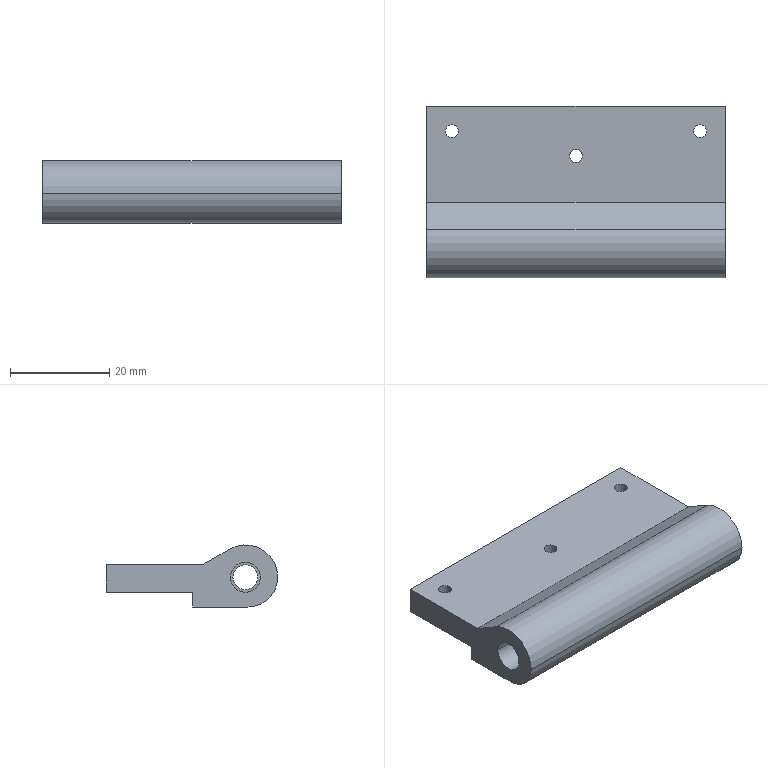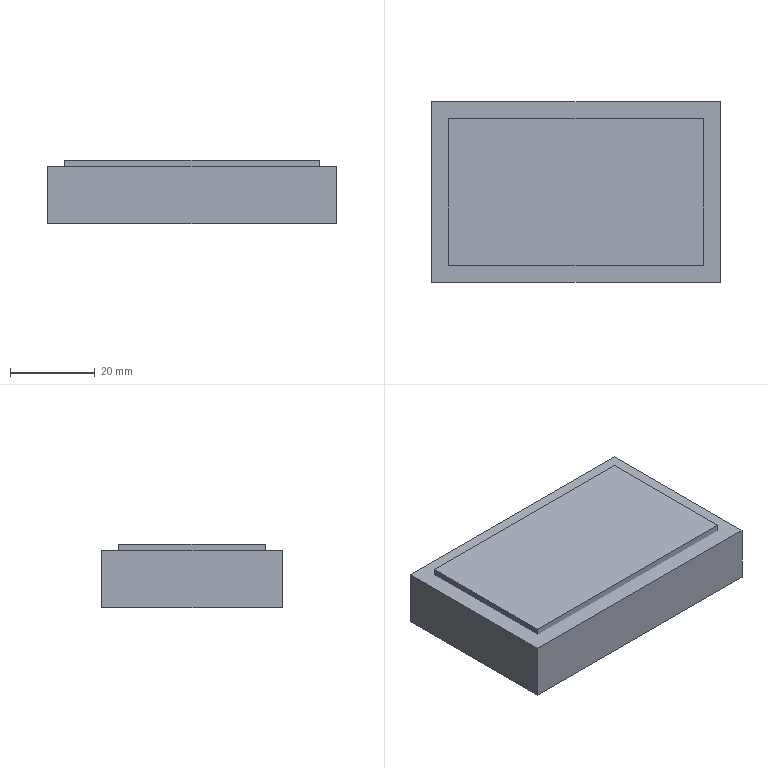CAM job | NX | 3+2 milling, drilling | part box 60 x 34.5 x 12.5 mm | stock box 68 x 42.5 x 15 mm
Tools:
number,name,description,diameter,corner_radius,flute_length,length,flutes
1,D63,Milling Tool-5 Parameters,63.0,0.0,50.0,75.0,2
10,D10,Milling Tool-5 Parameters,10.0,0.0,50.0,75.0,2
11,D10JING,Milling Tool-5 Parameters,10.0,0.0,50.0,75.0,2
7,D6A45,Milling Tool-5 Parameters,6.0,0.0,3.0,3.0,2
12,2.6ZT,Drilling Tool,2.6,0.0,35.0,50.0,2
5,D6R0.5,Milling Tool-5 Parameters,6.0,0.5,50.0,75.0,2
15,5.0ZT,Drilling Tool,5.0,0.0,35.0,50.0,2
4,D4,Milling Tool-5 Parameters,4.0,0.0,50.0,75.0,2
Operations:
program,operation,operation_type,tool,method,geometry_group,spindle_rpm,surface_speed,feed_per_tooth,feed_cut,feed_plunge,cut_length_mm,path_length_mm,cut_time_min,machine_time_min
1-65-40-15毛胚,FLOOR_WALL,VolumeBased25DMillingOperation,D63,METHOD,A,6500.0,1286.0,0.0962,1250.0,100.0,265.797,319.797,0.2126,0.218
1-65-40-15毛胚,ADAPTIVE_MILLING,CavityMilling,D10,METHOD,A,9500.0,298.0,0.1579,3000.0,1000.0,3662.408,4446.827,1.235,1.313
1-65-40-15毛胚,DRILLING_COPY_1,Operation,D6A45,METHOD,A,3500.0,43.0,0.0357,250.0,0.0,14.4,152.142,0.0576,0.0714
1-65-40-15毛胚,DRILLING_COPY_COPY_COPY_1,Operation,2.6ZT,METHOD,A,2500.0,19.0,0.024,120.0,0.0,32.343,188.029,0.2695,0.2851
1-65-40-15毛胚,ZLEVEL_PROFILE_1,ZLevelMilling,D10JING,METHOD,A,9500.0,298.0,0.0526,1000.0,100.0,229.412,311.412,0.2294,0.2376
1-65-40-15毛胚,FLOOR_WALL_1,VolumeBased25DMillingOperation,D10JING,METHOD,A,9500.0,298.0,0.0658,1250.0,100.0,385.899,506.399,0.3087,0.3208
1-65-40-15毛胚,ZLEVEL_PROFILE_COPY_COPY_1_COPY_1_COPY_1,ZLevelMilling,D6R0.5,METHOD,A,9500.0,179.0,0.1579,3000.0,1000.0,7075.717,7140.222,2.36,2.367
1-65-40-15毛胚,ZLEVEL_PROFILE_1_COPY_1_COPY_COPY_COPY_1_COPY_COPY_COPY,ZLevelMilling,D6A45,METHOD,A,9500.0,179.0,0.0526,1000.0,100.0,87.676,147.676,0.0877,0.0937
1-65-40-15毛胚,ZLEVEL_PROFILE_1_COPY_1_COPY_COPY_COPY_1_COPY_COPY_COPY_COPY,ZLevelMilling,D6A45,METHOD,A,9500.0,179.0,0.0526,1000.0,100.0,96.557,162.557,0.0966,0.1032
2,DRILLING_COPY_1_COPY,Operation,D6A45,METHOD,B,3500.0,43.0,0.0357,250.0,0.0,4.8,69.6,0.0192,0.0257
2,DRILLING_COPY_COPY_COPY_1_COPY,Operation,5.0ZT,METHOD,B,2000.0,31.0,0.025,100.0,0.0,56.202,172.404,0.562,0.5736
2,HOLE_MILLING,CylinderMilling,D4,METHOD,B,9500.0,89.0,0.0658,1250.0,100.0,244.371,313.671,0.1955,0.2024
2,ZLEVEL_PROFILE_1_COPY_1_COPY_COPY_COPY_1_COPY_COPY_COPY_COPY_1,ZLevelMilling,D6A45,METHOD,B,9500.0,179.0,0.0526,1000.0,100.0,18.097,78.097,0.0181,0.0241
2,CUTTERCOMP4,CylinderMilling,D4,METHOD,B,9500.0,89.0,0.0526,1000.0,100.0,41.796,111.096,0.0418,0.0487
3,HOLE_MILLING_COPY,CylinderMilling,D4,METHOD,C,9500.0,89.0,0.0658,1250.0,100.0,244.371,313.671,0.1955,0.2024
3,ZLEVEL_PROFILE_1_COPY_1_COPY_COPY_COPY_1_COPY_COPY_COPY_COPY_1_COPY,ZLevelMilling,D6A45,METHOD,C,9500.0,179.0,0.0526,1000.0,100.0,18.097,78.097,0.0181,0.0241
3,CUTTERCOMP4_COPY,CylinderMilling,D4,METHOD,C,9500.0,89.0,0.0526,1000.0,100.0,41.796,111.096,0.0418,0.0487
4,FACE_MILLING,FaceMilling,D63,METHOD,D,6500.0,1286.0,0.0962,1250.0,100.0,915.0,1154.0,0.732,0.7559
4,FLOOR_WALL_2,VolumeBased25DMillingOperation,D10,METHOD,D,9500.0,298.0,0.1053,2000.0,100.0,1225.701,1504.253,0.6129,0.6407
4,FLOOR_WALL_1_COPY,VolumeBased25DMillingOperation,D10JING,METHOD,D,9500.0,298.0,0.0658,1250.0,100.0,387.829,512.329,0.3103,0.3227
4,ZLEVEL_PROFILE_COPY_COPY_1_COPY_1_COPY_1_COPY,ZLevelMilling,D6R0.5,METHOD,D,9500.0,179.0,0.1579,3000.0,1000.0,17005.908,17215.957,5.678,5.699
4,ZLEVEL_PROFILE_1_COPY_1_COPY_COPY_COPY_1_COPY_COPY_COPY_COPY_COPY,ZLevelMilling,D6A45,METHOD,D,9500.0,179.0,0.0526,1000.0,100.0,120.575,500.384,0.1206,0.1586